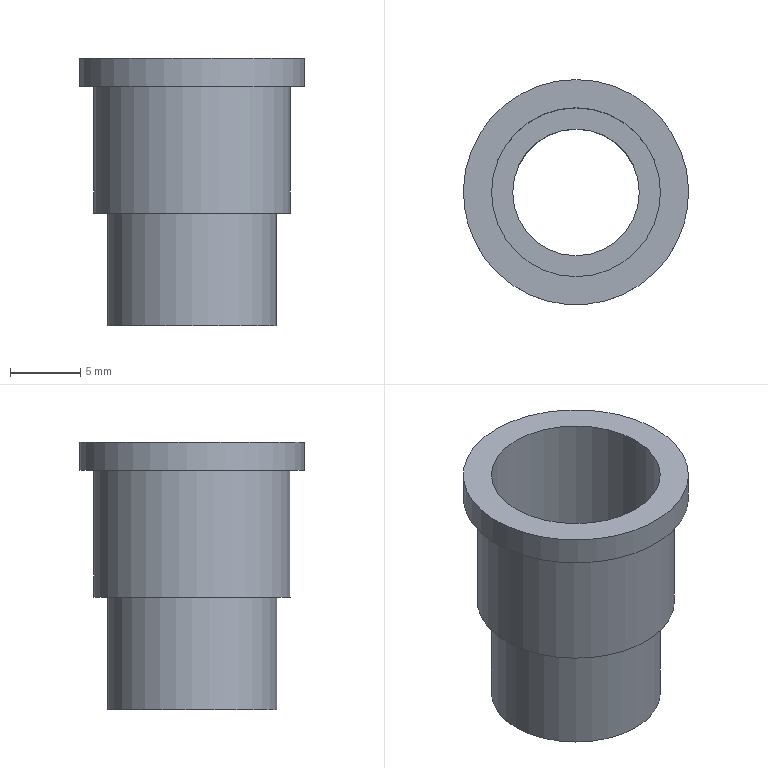Part | STEP file | 1-16.2 | 1 solid | 10 faces | box 16 x 16 x 19 mm | volume 1038 mm3 | cylinder 5 | plane 5 | commonest cylinder face diameters 12 x2 9 x1 14 x1 16 x1
STEP:
#1=CARTESIAN_POINT('',(0.,0.,0.));
#2=DIRECTION('',(0.,0.,1.));
#3=DIRECTION('',(1.,0.,0.));
#4=AXIS2_PLACEMENT_3D('',#1,#2,#3);
#5=CARTESIAN_POINT('',(0.,8.,0.));
#6=VERTEX_POINT('',#5);
#7=CARTESIAN_POINT('',(0.,0.,0.));
#8=DIRECTION('',(0.,0.,1.));
#9=DIRECTION('',(0.,1.,0.));
#10=AXIS2_PLACEMENT_3D('',#7,#8,#9);
#11=CIRCLE('',#10,8.);
#12=CARTESIAN_POINT('',(0.,0.,0.));
#13=DIRECTION('',(0.,0.,1.));
#14=DIRECTION('',(0.,1.,0.));
#15=AXIS2_PLACEMENT_3D('',#12,#13,#14);
#16=CYLINDRICAL_SURFACE('',#15,8.);
#17=CARTESIAN_POINT('',(0.,0.));
#18=DIRECTION('',(1.,0.));
#19=VECTOR('',#18,1.);
#20=LINE('',#17,#19);
#21=(GEOMETRIC_REPRESENTATION_CONTEXT(2)PARAMETRIC_REPRESENTATION_CONTEXT()REPRESENTATION_CONTEXT('',''));
#22=DEFINITIONAL_REPRESENTATION('',(#20),#21);
#23=PCURVE('',#16,#22);
#24=CARTESIAN_POINT('',(0.,-2.144,0.));
#25=DIRECTION('',(0.,0.,1.));
#26=DIRECTION('',(1.,0.,0.));
#27=AXIS2_PLACEMENT_3D('',#24,#25,#26);
#28=PLANE('',#27);
#29=CARTESIAN_POINT('',(0.,2.144));
#30=DIRECTION('',(0.,1.));
#31=AXIS2_PLACEMENT_2D('',#29,#30);
#32=CIRCLE('',#31,8.);
#33=(GEOMETRIC_REPRESENTATION_CONTEXT(2)PARAMETRIC_REPRESENTATION_CONTEXT()REPRESENTATION_CONTEXT('',''));
#34=DEFINITIONAL_REPRESENTATION('',(#32),#33);
#35=PCURVE('',#28,#34);
#36=SURFACE_CURVE('',#11,(#23,#35),.PCURVE_S1.);
#37=EDGE_CURVE('',#6,#6,#36,.T.);
#38=ORIENTED_EDGE('',*,*,#37,.T.);
#39=CARTESIAN_POINT('',(0.,8.,2.));
#40=VERTEX_POINT('',#39);
#41=CARTESIAN_POINT('',(0.,8.,0.));
#42=DIRECTION('',(0.,0.,1.));
#43=VECTOR('',#42,1.);
#44=LINE('',#41,#43);
#45=CARTESIAN_POINT('',(6.283,0.));
#46=DIRECTION('',(0.,1.));
#47=VECTOR('',#46,1.);
#48=LINE('',#45,#47);
#49=(GEOMETRIC_REPRESENTATION_CONTEXT(2)PARAMETRIC_REPRESENTATION_CONTEXT()REPRESENTATION_CONTEXT('',''));
#50=DEFINITIONAL_REPRESENTATION('',(#48),#49);
#51=PCURVE('',#16,#50);
#52=CARTESIAN_POINT('',(0.,0.));
#53=DIRECTION('',(0.,1.));
#54=VECTOR('',#53,1.);
#55=LINE('',#52,#54);
#56=(GEOMETRIC_REPRESENTATION_CONTEXT(2)PARAMETRIC_REPRESENTATION_CONTEXT()REPRESENTATION_CONTEXT('',''));
#57=DEFINITIONAL_REPRESENTATION('',(#55),#56);
#58=PCURVE('',#16,#57);
#59=SEAM_CURVE('',#44,(#51,#58),.PCURVE_S1.);
#60=EDGE_CURVE('',#6,#40,#59,.T.);
#61=ORIENTED_EDGE('',*,*,#60,.T.);
#62=CARTESIAN_POINT('',(0.,0.,2.));
#63=DIRECTION('',(0.,0.,1.));
#64=DIRECTION('',(0.,1.,0.));
#65=AXIS2_PLACEMENT_3D('',#62,#63,#64);
#66=CIRCLE('',#65,8.);
#67=CARTESIAN_POINT('',(0.,2.));
#68=DIRECTION('',(1.,0.));
#69=VECTOR('',#68,1.);
#70=LINE('',#67,#69);
#71=(GEOMETRIC_REPRESENTATION_CONTEXT(2)PARAMETRIC_REPRESENTATION_CONTEXT()REPRESENTATION_CONTEXT('',''));
#72=DEFINITIONAL_REPRESENTATION('',(#70),#71);
#73=PCURVE('',#16,#72);
#74=CARTESIAN_POINT('',(0.,-2.144,2.));
#75=DIRECTION('',(0.,0.,1.));
#76=DIRECTION('',(1.,0.,0.));
#77=AXIS2_PLACEMENT_3D('',#74,#75,#76);
#78=PLANE('',#77);
#79=CARTESIAN_POINT('',(0.,2.144));
#80=DIRECTION('',(0.,1.));
#81=AXIS2_PLACEMENT_2D('',#79,#80);
#82=CIRCLE('',#81,8.);
#83=(GEOMETRIC_REPRESENTATION_CONTEXT(2)PARAMETRIC_REPRESENTATION_CONTEXT()REPRESENTATION_CONTEXT('',''));
#84=DEFINITIONAL_REPRESENTATION('',(#82),#83);
#85=PCURVE('',#78,#84);
#86=SURFACE_CURVE('',#66,(#73,#85),.PCURVE_S1.);
#87=EDGE_CURVE('',#40,#40,#86,.T.);
#88=ORIENTED_EDGE('',*,*,#87,.F.);
#89=ORIENTED_EDGE('',*,*,#60,.F.);
#90=EDGE_LOOP('',(#38,#61,#88,#89));
#91=FACE_BOUND('',#90,.T.);
#92=ADVANCED_FACE('',(#91),#16,.T.);
#93=ORIENTED_EDGE('',*,*,#37,.T.);
#94=EDGE_LOOP('',(#93));
#95=FACE_BOUND('',#94,.F.);
#96=CARTESIAN_POINT('',(0.,7.,0.));
#97=VERTEX_POINT('',#96);
#98=CARTESIAN_POINT('',(0.,0.,0.));
#99=DIRECTION('',(0.,0.,1.));
#100=DIRECTION('',(0.,1.,0.));
#101=AXIS2_PLACEMENT_3D('',#98,#99,#100);
#102=CIRCLE('',#101,7.);
#103=CARTESIAN_POINT('',(0.,2.144));
#104=DIRECTION('',(0.,1.));
#105=AXIS2_PLACEMENT_2D('',#103,#104);
#106=CIRCLE('',#105,7.);
#107=(GEOMETRIC_REPRESENTATION_CONTEXT(2)PARAMETRIC_REPRESENTATION_CONTEXT()REPRESENTATION_CONTEXT('',''));
#108=DEFINITIONAL_REPRESENTATION('',(#106),#107);
#109=PCURVE('',#28,#108);
#110=CARTESIAN_POINT('',(0.,0.,0.));
#111=DIRECTION('',(0.,0.,-1.));
#112=DIRECTION('',(0.,1.,0.));
#113=AXIS2_PLACEMENT_3D('',#110,#111,#112);
#114=CYLINDRICAL_SURFACE('',#113,7.);
#115=CARTESIAN_POINT('',(6.283,0.));
#116=DIRECTION('',(-1.,0.));
#117=VECTOR('',#116,1.);
#118=LINE('',#115,#117);
#119=(GEOMETRIC_REPRESENTATION_CONTEXT(2)PARAMETRIC_REPRESENTATION_CONTEXT()REPRESENTATION_CONTEXT('',''));
#120=DEFINITIONAL_REPRESENTATION('',(#118),#119);
#121=PCURVE('',#114,#120);
#122=SURFACE_CURVE('',#102,(#109,#121),.PCURVE_S1.);
#123=EDGE_CURVE('',#97,#97,#122,.T.);
#124=ORIENTED_EDGE('',*,*,#123,.F.);
#125=EDGE_LOOP('',(#124));
#126=FACE_BOUND('',#125,.F.);
#127=ADVANCED_FACE('',(#95,#126),#28,.F.);
#128=CARTESIAN_POINT('',(0.,7.,-9.));
#129=VERTEX_POINT('',#128);
#130=CARTESIAN_POINT('',(0.,7.,0.));
#131=DIRECTION('',(0.,0.,-1.));
#132=VECTOR('',#131,1.);
#133=LINE('',#130,#132);
#134=CARTESIAN_POINT('',(6.283,0.));
#135=DIRECTION('',(0.,1.));
#136=VECTOR('',#135,1.);
#137=LINE('',#134,#136);
#138=(GEOMETRIC_REPRESENTATION_CONTEXT(2)PARAMETRIC_REPRESENTATION_CONTEXT()REPRESENTATION_CONTEXT('',''));
#139=DEFINITIONAL_REPRESENTATION('',(#137),#138);
#140=PCURVE('',#114,#139);
#141=CARTESIAN_POINT('',(0.,0.));
#142=DIRECTION('',(0.,1.));
#143=VECTOR('',#142,1.);
#144=LINE('',#141,#143);
#145=(GEOMETRIC_REPRESENTATION_CONTEXT(2)PARAMETRIC_REPRESENTATION_CONTEXT()REPRESENTATION_CONTEXT('',''));
#146=DEFINITIONAL_REPRESENTATION('',(#144),#145);
#147=PCURVE('',#114,#146);
#148=SEAM_CURVE('',#133,(#140,#147),.PCURVE_S1.);
#149=EDGE_CURVE('',#97,#129,#148,.T.);
#150=ORIENTED_EDGE('',*,*,#149,.T.);
#151=CARTESIAN_POINT('',(0.,0.,-9.));
#152=DIRECTION('',(0.,0.,1.));
#153=DIRECTION('',(0.,1.,0.));
#154=AXIS2_PLACEMENT_3D('',#151,#152,#153);
#155=CIRCLE('',#154,7.);
#156=CARTESIAN_POINT('',(6.283,9.));
#157=DIRECTION('',(-1.,0.));
#158=VECTOR('',#157,1.);
#159=LINE('',#156,#158);
#160=(GEOMETRIC_REPRESENTATION_CONTEXT(2)PARAMETRIC_REPRESENTATION_CONTEXT()REPRESENTATION_CONTEXT('',''));
#161=DEFINITIONAL_REPRESENTATION('',(#159),#160);
#162=PCURVE('',#114,#161);
#163=CARTESIAN_POINT('',(0.,-1.876,-9.));
#164=DIRECTION('',(0.,0.,1.));
#165=DIRECTION('',(1.,0.,0.));
#166=AXIS2_PLACEMENT_3D('',#163,#164,#165);
#167=PLANE('',#166);
#168=CARTESIAN_POINT('',(0.,1.876));
#169=DIRECTION('',(0.,1.));
#170=AXIS2_PLACEMENT_2D('',#168,#169);
#171=CIRCLE('',#170,7.);
#172=(GEOMETRIC_REPRESENTATION_CONTEXT(2)PARAMETRIC_REPRESENTATION_CONTEXT()REPRESENTATION_CONTEXT('',''));
#173=DEFINITIONAL_REPRESENTATION('',(#171),#172);
#174=PCURVE('',#167,#173);
#175=SURFACE_CURVE('',#155,(#162,#174),.PCURVE_S1.);
#176=EDGE_CURVE('',#129,#129,#175,.T.);
#177=ORIENTED_EDGE('',*,*,#176,.T.);
#178=ORIENTED_EDGE('',*,*,#149,.F.);
#179=ORIENTED_EDGE('',*,*,#123,.F.);
#180=EDGE_LOOP('',(#150,#177,#178,#179));
#181=FACE_BOUND('',#180,.T.);
#182=ADVANCED_FACE('',(#181),#114,.T.);
#183=ORIENTED_EDGE('',*,*,#176,.T.);
#184=EDGE_LOOP('',(#183));
#185=FACE_BOUND('',#184,.F.);
#186=CARTESIAN_POINT('',(0.,6.,-9.));
#187=VERTEX_POINT('',#186);
#188=CARTESIAN_POINT('',(0.,0.,-9.));
#189=DIRECTION('',(0.,0.,-1.));
#190=DIRECTION('',(0.,1.,0.));
#191=AXIS2_PLACEMENT_3D('',#188,#189,#190);
#192=CIRCLE('',#191,6.);
#193=CARTESIAN_POINT('',(0.,7.876));
#194=CARTESIAN_POINT('',(10.392,7.876));
#195=CARTESIAN_POINT('',(5.196,-1.124));
#196=CARTESIAN_POINT('',(0.,-10.124));
#197=CARTESIAN_POINT('',(-5.196,-1.124));
#198=CARTESIAN_POINT('',(-10.392,7.876));
#199=CARTESIAN_POINT('',(0.,7.876));
#200=(BOUNDED_CURVE()B_SPLINE_CURVE(2,(#193,#194,#195,#196,#197,#198,#199),.UNSPECIFIED.,.T.,.F.)B_SPLINE_CURVE_WITH_KNOTS((1,2,2,2,2,1),(-2.094,0.,2.094,4.189,6.283,8.378),.UNSPECIFIED.)CURVE()GEOMETRIC_REPRESENTATION_ITEM()RATIONAL_B_SPLINE_CURVE((1.,0.5,1.,0.5,1.,0.5,1.))REPRESENTATION_ITEM(''));
#201=(GEOMETRIC_REPRESENTATION_CONTEXT(2)PARAMETRIC_REPRESENTATION_CONTEXT()REPRESENTATION_CONTEXT('',''));
#202=DEFINITIONAL_REPRESENTATION('',(#200),#201);
#203=PCURVE('',#167,#202);
#204=CARTESIAN_POINT('',(0.,0.,-9.));
#205=DIRECTION('',(0.,0.,-1.));
#206=DIRECTION('',(0.,1.,0.));
#207=AXIS2_PLACEMENT_3D('',#204,#205,#206);
#208=CYLINDRICAL_SURFACE('',#207,6.);
#209=CARTESIAN_POINT('',(0.,0.));
#210=DIRECTION('',(1.,0.));
#211=VECTOR('',#210,1.);
#212=LINE('',#209,#211);
#213=(GEOMETRIC_REPRESENTATION_CONTEXT(2)PARAMETRIC_REPRESENTATION_CONTEXT()REPRESENTATION_CONTEXT('',''));
#214=DEFINITIONAL_REPRESENTATION('',(#212),#213);
#215=PCURVE('',#208,#214);
#216=SURFACE_CURVE('',#192,(#203,#215),.PCURVE_S1.);
#217=EDGE_CURVE('',#187,#187,#216,.T.);
#218=ORIENTED_EDGE('',*,*,#217,.T.);
#219=EDGE_LOOP('',(#218));
#220=FACE_BOUND('',#219,.F.);
#221=ADVANCED_FACE('',(#185,#220),#167,.F.);
#222=ORIENTED_EDGE('',*,*,#217,.T.);
#223=CARTESIAN_POINT('',(0.,6.,-17.));
#224=VERTEX_POINT('',#223);
#225=CARTESIAN_POINT('',(0.,6.,-9.));
#226=DIRECTION('',(0.,0.,-1.));
#227=VECTOR('',#226,1.);
#228=LINE('',#225,#227);
#229=CARTESIAN_POINT('',(6.283,0.));
#230=DIRECTION('',(0.,1.));
#231=VECTOR('',#230,1.);
#232=LINE('',#229,#231);
#233=(GEOMETRIC_REPRESENTATION_CONTEXT(2)PARAMETRIC_REPRESENTATION_CONTEXT()REPRESENTATION_CONTEXT('',''));
#234=DEFINITIONAL_REPRESENTATION('',(#232),#233);
#235=PCURVE('',#208,#234);
#236=CARTESIAN_POINT('',(0.,0.));
#237=DIRECTION('',(0.,1.));
#238=VECTOR('',#237,1.);
#239=LINE('',#236,#238);
#240=(GEOMETRIC_REPRESENTATION_CONTEXT(2)PARAMETRIC_REPRESENTATION_CONTEXT()REPRESENTATION_CONTEXT('',''));
#241=DEFINITIONAL_REPRESENTATION('',(#239),#240);
#242=PCURVE('',#208,#241);
#243=SEAM_CURVE('',#228,(#235,#242),.PCURVE_S1.);
#244=EDGE_CURVE('',#187,#224,#243,.T.);
#245=ORIENTED_EDGE('',*,*,#244,.T.);
#246=CARTESIAN_POINT('',(0.,0.,-17.));
#247=DIRECTION('',(0.,0.,-1.));
#248=DIRECTION('',(0.,1.,0.));
#249=AXIS2_PLACEMENT_3D('',#246,#247,#248);
#250=CIRCLE('',#249,6.);
#251=CARTESIAN_POINT('',(0.,8.));
#252=DIRECTION('',(1.,0.));
#253=VECTOR('',#252,1.);
#254=LINE('',#251,#253);
#255=(GEOMETRIC_REPRESENTATION_CONTEXT(2)PARAMETRIC_REPRESENTATION_CONTEXT()REPRESENTATION_CONTEXT('',''));
#256=DEFINITIONAL_REPRESENTATION('',(#254),#255);
#257=PCURVE('',#208,#256);
#258=CARTESIAN_POINT('',(0.,-1.608,-17.));
#259=DIRECTION('',(0.,0.,-1.));
#260=DIRECTION('',(0.,1.,0.));
#261=AXIS2_PLACEMENT_3D('',#258,#259,#260);
#262=PLANE('',#261);
#263=CARTESIAN_POINT('',(1.608,0.));
#264=DIRECTION('',(1.,0.));
#265=AXIS2_PLACEMENT_2D('',#263,#264);
#266=CIRCLE('',#265,6.);
#267=(GEOMETRIC_REPRESENTATION_CONTEXT(2)PARAMETRIC_REPRESENTATION_CONTEXT()REPRESENTATION_CONTEXT('',''));
#268=DEFINITIONAL_REPRESENTATION('',(#266),#267);
#269=PCURVE('',#262,#268);
#270=SURFACE_CURVE('',#250,(#257,#269),.PCURVE_S1.);
#271=EDGE_CURVE('',#224,#224,#270,.T.);
#272=ORIENTED_EDGE('',*,*,#271,.F.);
#273=ORIENTED_EDGE('',*,*,#244,.F.);
#274=EDGE_LOOP('',(#222,#245,#272,#273));
#275=FACE_BOUND('',#274,.T.);
#276=ADVANCED_FACE('',(#275),#208,.T.);
#277=ORIENTED_EDGE('',*,*,#87,.T.);
#278=EDGE_LOOP('',(#277));
#279=FACE_BOUND('',#278,.T.);
#280=CARTESIAN_POINT('',(0.,6.,2.));
#281=VERTEX_POINT('',#280);
#282=CARTESIAN_POINT('',(0.,0.,2.));
#283=DIRECTION('',(0.,0.,1.));
#284=DIRECTION('',(0.,1.,0.));
#285=AXIS2_PLACEMENT_3D('',#282,#283,#284);
#286=CIRCLE('',#285,6.);
#287=CARTESIAN_POINT('',(0.,2.144));
#288=DIRECTION('',(0.,1.));
#289=AXIS2_PLACEMENT_2D('',#287,#288);
#290=CIRCLE('',#289,6.);
#291=(GEOMETRIC_REPRESENTATION_CONTEXT(2)PARAMETRIC_REPRESENTATION_CONTEXT()REPRESENTATION_CONTEXT('',''));
#292=DEFINITIONAL_REPRESENTATION('',(#290),#291);
#293=PCURVE('',#78,#292);
#294=CARTESIAN_POINT('',(0.,0.,2.));
#295=DIRECTION('',(0.,0.,-1.));
#296=DIRECTION('',(0.,1.,0.));
#297=AXIS2_PLACEMENT_3D('',#294,#295,#296);
#298=CYLINDRICAL_SURFACE('',#297,6.);
#299=CARTESIAN_POINT('',(6.283,0.));
#300=DIRECTION('',(-1.,0.));
#301=VECTOR('',#300,1.);
#302=LINE('',#299,#301);
#303=(GEOMETRIC_REPRESENTATION_CONTEXT(2)PARAMETRIC_REPRESENTATION_CONTEXT()REPRESENTATION_CONTEXT('',''));
#304=DEFINITIONAL_REPRESENTATION('',(#302),#303);
#305=PCURVE('',#298,#304);
#306=SURFACE_CURVE('',#286,(#293,#305),.PCURVE_S1.);
#307=EDGE_CURVE('',#281,#281,#306,.T.);
#308=ORIENTED_EDGE('',*,*,#307,.F.);
#309=EDGE_LOOP('',(#308));
#310=FACE_BOUND('',#309,.T.);
#311=ADVANCED_FACE('',(#279,#310),#78,.T.);
#312=CARTESIAN_POINT('',(0.,6.,-7.));
#313=VERTEX_POINT('',#312);
#314=CARTESIAN_POINT('',(0.,6.,2.));
#315=DIRECTION('',(0.,0.,-1.));
#316=VECTOR('',#315,1.);
#317=LINE('',#314,#316);
#318=CARTESIAN_POINT('',(6.283,0.));
#319=DIRECTION('',(0.,1.));
#320=VECTOR('',#319,1.);
#321=LINE('',#318,#320);
#322=(GEOMETRIC_REPRESENTATION_CONTEXT(2)PARAMETRIC_REPRESENTATION_CONTEXT()REPRESENTATION_CONTEXT('',''));
#323=DEFINITIONAL_REPRESENTATION('',(#321),#322);
#324=PCURVE('',#298,#323);
#325=CARTESIAN_POINT('',(0.,0.));
#326=DIRECTION('',(0.,1.));
#327=VECTOR('',#326,1.);
#328=LINE('',#325,#327);
#329=(GEOMETRIC_REPRESENTATION_CONTEXT(2)PARAMETRIC_REPRESENTATION_CONTEXT()REPRESENTATION_CONTEXT('',''));
#330=DEFINITIONAL_REPRESENTATION('',(#328),#329);
#331=PCURVE('',#298,#330);
#332=SEAM_CURVE('',#317,(#324,#331),.PCURVE_S1.);
#333=EDGE_CURVE('',#281,#313,#332,.T.);
#334=ORIENTED_EDGE('',*,*,#333,.T.);
#335=CARTESIAN_POINT('',(0.,0.,-7.));
#336=DIRECTION('',(0.,0.,1.));
#337=DIRECTION('',(0.,1.,0.));
#338=AXIS2_PLACEMENT_3D('',#335,#336,#337);
#339=CIRCLE('',#338,6.);
#340=CARTESIAN_POINT('',(6.283,9.));
#341=DIRECTION('',(-1.,0.));
#342=VECTOR('',#341,1.);
#343=LINE('',#340,#342);
#344=(GEOMETRIC_REPRESENTATION_CONTEXT(2)PARAMETRIC_REPRESENTATION_CONTEXT()REPRESENTATION_CONTEXT('',''));
#345=DEFINITIONAL_REPRESENTATION('',(#343),#344);
#346=PCURVE('',#298,#345);
#347=CARTESIAN_POINT('',(0.,-1.608,-7.));
#348=DIRECTION('',(0.,0.,1.));
#349=DIRECTION('',(0.,1.,0.));
#350=AXIS2_PLACEMENT_3D('',#347,#348,#349);
#351=PLANE('',#350);
#352=CARTESIAN_POINT('',(1.608,0.));
#353=DIRECTION('',(1.,0.));
#354=AXIS2_PLACEMENT_2D('',#352,#353);
#355=CIRCLE('',#354,6.);
#356=(GEOMETRIC_REPRESENTATION_CONTEXT(2)PARAMETRIC_REPRESENTATION_CONTEXT()REPRESENTATION_CONTEXT('',''));
#357=DEFINITIONAL_REPRESENTATION('',(#355),#356);
#358=PCURVE('',#351,#357);
#359=SURFACE_CURVE('',#339,(#346,#358),.PCURVE_S1.);
#360=EDGE_CURVE('',#313,#313,#359,.T.);
#361=ORIENTED_EDGE('',*,*,#360,.T.);
#362=ORIENTED_EDGE('',*,*,#333,.F.);
#363=ORIENTED_EDGE('',*,*,#307,.F.);
#364=EDGE_LOOP('',(#334,#361,#362,#363));
#365=FACE_BOUND('',#364,.F.);
#366=ADVANCED_FACE('',(#365),#298,.F.);
#367=ORIENTED_EDGE('',*,*,#271,.T.);
#368=EDGE_LOOP('',(#367));
#369=FACE_BOUND('',#368,.T.);
#370=CARTESIAN_POINT('',(0.,4.5,-17.));
#371=VERTEX_POINT('',#370);
#372=CARTESIAN_POINT('',(0.,0.,-17.));
#373=DIRECTION('',(0.,0.,1.));
#374=DIRECTION('',(0.,1.,0.));
#375=AXIS2_PLACEMENT_3D('',#372,#373,#374);
#376=CIRCLE('',#375,4.5);
#377=CARTESIAN_POINT('',(6.108,0.));
#378=CARTESIAN_POINT('',(6.108,-7.794));
#379=CARTESIAN_POINT('',(-0.6423,-3.897));
#380=CARTESIAN_POINT('',(-7.392,0.));
#381=CARTESIAN_POINT('',(-0.6423,3.897));
#382=CARTESIAN_POINT('',(6.108,7.794));
#383=CARTESIAN_POINT('',(6.108,0.));
#384=(BOUNDED_CURVE()B_SPLINE_CURVE(2,(#377,#378,#379,#380,#381,#382,#383),.UNSPECIFIED.,.T.,.F.)B_SPLINE_CURVE_WITH_KNOTS((1,2,2,2,2,1),(-2.094,0.,2.094,4.189,6.283,8.378),.UNSPECIFIED.)CURVE()GEOMETRIC_REPRESENTATION_ITEM()RATIONAL_B_SPLINE_CURVE((1.,0.5,1.,0.5,1.,0.5,1.))REPRESENTATION_ITEM(''));
#385=(GEOMETRIC_REPRESENTATION_CONTEXT(2)PARAMETRIC_REPRESENTATION_CONTEXT()REPRESENTATION_CONTEXT('',''));
#386=DEFINITIONAL_REPRESENTATION('',(#384),#385);
#387=PCURVE('',#262,#386);
#388=CARTESIAN_POINT('',(0.,0.,-7.));
#389=DIRECTION('',(0.,0.,-1.));
#390=DIRECTION('',(0.,1.,0.));
#391=AXIS2_PLACEMENT_3D('',#388,#389,#390);
#392=CYLINDRICAL_SURFACE('',#391,4.5);
#393=CARTESIAN_POINT('',(6.283,10.));
#394=DIRECTION('',(-1.,0.));
#395=VECTOR('',#394,1.);
#396=LINE('',#393,#395);
#397=(GEOMETRIC_REPRESENTATION_CONTEXT(2)PARAMETRIC_REPRESENTATION_CONTEXT()REPRESENTATION_CONTEXT('',''));
#398=DEFINITIONAL_REPRESENTATION('',(#396),#397);
#399=PCURVE('',#392,#398);
#400=SURFACE_CURVE('',#376,(#387,#399),.PCURVE_S1.);
#401=EDGE_CURVE('',#371,#371,#400,.T.);
#402=ORIENTED_EDGE('',*,*,#401,.T.);
#403=EDGE_LOOP('',(#402));
#404=FACE_BOUND('',#403,.T.);
#405=ADVANCED_FACE('',(#369,#404),#262,.T.);
#406=ORIENTED_EDGE('',*,*,#360,.T.);
#407=EDGE_LOOP('',(#406));
#408=FACE_BOUND('',#407,.T.);
#409=CARTESIAN_POINT('',(0.,4.5,-7.));
#410=VERTEX_POINT('',#409);
#411=CARTESIAN_POINT('',(0.,0.,-7.));
#412=DIRECTION('',(0.,0.,1.));
#413=DIRECTION('',(0.,1.,0.));
#414=AXIS2_PLACEMENT_3D('',#411,#412,#413);
#415=CIRCLE('',#414,4.5);
#416=CARTESIAN_POINT('',(1.608,0.));
#417=DIRECTION('',(1.,0.));
#418=AXIS2_PLACEMENT_2D('',#416,#417);
#419=CIRCLE('',#418,4.5);
#420=(GEOMETRIC_REPRESENTATION_CONTEXT(2)PARAMETRIC_REPRESENTATION_CONTEXT()REPRESENTATION_CONTEXT('',''));
#421=DEFINITIONAL_REPRESENTATION('',(#419),#420);
#422=PCURVE('',#351,#421);
#423=CARTESIAN_POINT('',(6.283,0.));
#424=DIRECTION('',(-1.,0.));
#425=VECTOR('',#424,1.);
#426=LINE('',#423,#425);
#427=(GEOMETRIC_REPRESENTATION_CONTEXT(2)PARAMETRIC_REPRESENTATION_CONTEXT()REPRESENTATION_CONTEXT('',''));
#428=DEFINITIONAL_REPRESENTATION('',(#426),#427);
#429=PCURVE('',#392,#428);
#430=SURFACE_CURVE('',#415,(#422,#429),.PCURVE_S1.);
#431=EDGE_CURVE('',#410,#410,#430,.T.);
#432=ORIENTED_EDGE('',*,*,#431,.F.);
#433=EDGE_LOOP('',(#432));
#434=FACE_BOUND('',#433,.T.);
#435=ADVANCED_FACE('',(#408,#434),#351,.T.);
#436=CARTESIAN_POINT('',(0.,4.5,-7.));
#437=DIRECTION('',(0.,0.,-1.));
#438=VECTOR('',#437,1.);
#439=LINE('',#436,#438);
#440=CARTESIAN_POINT('',(6.283,0.));
#441=DIRECTION('',(0.,1.));
#442=VECTOR('',#441,1.);
#443=LINE('',#440,#442);
#444=(GEOMETRIC_REPRESENTATION_CONTEXT(2)PARAMETRIC_REPRESENTATION_CONTEXT()REPRESENTATION_CONTEXT('',''));
#445=DEFINITIONAL_REPRESENTATION('',(#443),#444);
#446=PCURVE('',#392,#445);
#447=CARTESIAN_POINT('',(0.,0.));
#448=DIRECTION('',(0.,1.));
#449=VECTOR('',#448,1.);
#450=LINE('',#447,#449);
#451=(GEOMETRIC_REPRESENTATION_CONTEXT(2)PARAMETRIC_REPRESENTATION_CONTEXT()REPRESENTATION_CONTEXT('',''));
#452=DEFINITIONAL_REPRESENTATION('',(#450),#451);
#453=PCURVE('',#392,#452);
#454=SEAM_CURVE('',#439,(#446,#453),.PCURVE_S1.);
#455=EDGE_CURVE('',#410,#371,#454,.T.);
#456=ORIENTED_EDGE('',*,*,#455,.T.);
#457=ORIENTED_EDGE('',*,*,#401,.T.);
#458=ORIENTED_EDGE('',*,*,#455,.F.);
#459=ORIENTED_EDGE('',*,*,#431,.F.);
#460=EDGE_LOOP('',(#456,#457,#458,#459));
#461=FACE_BOUND('',#460,.F.);
#462=ADVANCED_FACE('',(#461),#392,.F.);
#463=CLOSED_SHELL('',(#92,#127,#182,#221,#276,#311,#366,#405,#435,#462));
#464=MANIFOLD_SOLID_BREP('',#463);
#465=(LENGTH_UNIT()NAMED_UNIT(*)SI_UNIT(.MILLI.,.METRE.));
#466=UNCERTAINTY_MEASURE_WITH_UNIT(LENGTH_MEASURE(0.0000001),#465,'','');
#467=(NAMED_UNIT(*)PLANE_ANGLE_UNIT()SI_UNIT($,.RADIAN.));
#468=(NAMED_UNIT(*)SI_UNIT($,.STERADIAN.)SOLID_ANGLE_UNIT());
#469=(GEOMETRIC_REPRESENTATION_CONTEXT(3)GLOBAL_UNCERTAINTY_ASSIGNED_CONTEXT((#466))GLOBAL_UNIT_ASSIGNED_CONTEXT((#465,#467,#468))REPRESENTATION_CONTEXT('',''));
#470=ADVANCED_BREP_SHAPE_REPRESENTATION('',(#4,#464),#469);